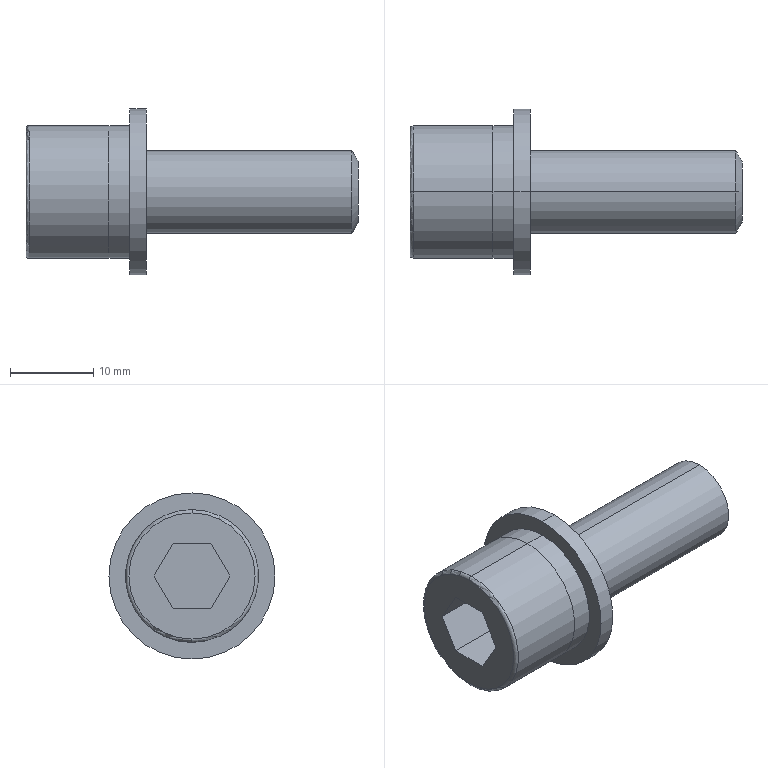Part | SolidWorks | features BaseBody 3 | 3 solids | 36 faces | box 40 x 20 x 20 mm | volume 4745 mm3 | plane 16 | cylinder 14 | torus 4 | cone 2 | commonest cylinder face diameters 16 x5 11 x3 10 x2 10.5 x2 20 x2
STEP:
#1=CARTESIAN_POINT('',(40.,0.,3.701));
#2=VERTEX_POINT('',#1);
#3=CARTESIAN_POINT('',(40.,0.,-3.701));
#4=VERTEX_POINT('',#3);
#5=CARTESIAN_POINT('',(40.,0.,0.));
#6=DIRECTION('',(-1.,0.,0.));
#7=DIRECTION('',(0.,0.,1.));
#8=AXIS2_PLACEMENT_3D('',#5,#6,#7);
#9=CIRCLE('',#8,3.701);
#10=EDGE_CURVE('',#2,#4,#9,.T.);
#11=ORIENTED_EDGE('',*,*,#10,.T.);
#12=CARTESIAN_POINT('',(39.25,0.,-5.));
#13=VERTEX_POINT('',#12);
#14=CARTESIAN_POINT('',(39.25,0.,-5.));
#15=DIRECTION('',(-0.5,0.,-0.866));
#16=VECTOR('',#15,1000.);
#17=LINE('',#14,#16);
#18=EDGE_CURVE('',#4,#13,#17,.T.);
#19=ORIENTED_EDGE('',*,*,#18,.T.);
#20=CARTESIAN_POINT('',(39.25,0.,5.));
#21=VERTEX_POINT('',#20);
#22=CARTESIAN_POINT('',(39.25,0.,0.));
#23=DIRECTION('',(-1.,0.,0.));
#24=DIRECTION('',(0.,0.,1.));
#25=AXIS2_PLACEMENT_3D('',#22,#23,#24);
#26=CIRCLE('',#25,5.);
#27=EDGE_CURVE('',#21,#13,#26,.T.);
#28=ORIENTED_EDGE('',*,*,#27,.F.);
#29=CARTESIAN_POINT('',(39.25,0.,5.));
#30=DIRECTION('',(-0.5,0.,0.866));
#31=VECTOR('',#30,1000.);
#32=LINE('',#29,#31);
#33=EDGE_CURVE('',#2,#21,#32,.T.);
#34=ORIENTED_EDGE('',*,*,#33,.F.);
#35=EDGE_LOOP('',(#11,#19,#28,#34));
#36=FACE_OUTER_BOUND('',#35,.T.);
#37=CARTESIAN_POINT('',(39.25,0.,0.));
#38=DIRECTION('',(-1.,0.,0.));
#39=DIRECTION('',(0.,0.,1.));
#40=AXIS2_PLACEMENT_3D('',#37,#38,#39);
#41=CONICAL_SURFACE('',#40,5.,1.047);
#42=ADVANCED_FACE('',(#36),#41,.T.);
#43=CARTESIAN_POINT('',(0.4,0.,-8.));
#44=VERTEX_POINT('',#43);
#45=CARTESIAN_POINT('',(0.4,0.,8.));
#46=VERTEX_POINT('',#45);
#47=CARTESIAN_POINT('',(0.4,0.,0.));
#48=DIRECTION('',(1.,0.,0.));
#49=DIRECTION('',(0.,0.,1.));
#50=AXIS2_PLACEMENT_3D('',#47,#48,#49);
#51=CIRCLE('',#50,8.);
#52=EDGE_CURVE('',#44,#46,#51,.T.);
#53=ORIENTED_EDGE('',*,*,#52,.F.);
#54=CARTESIAN_POINT('',(0.,0.,-7.6));
#55=VERTEX_POINT('',#54);
#56=CARTESIAN_POINT('',(0.4,0.,-7.6));
#57=DIRECTION('',(0.,1.,0.));
#58=DIRECTION('',(0.,0.,1.));
#59=AXIS2_PLACEMENT_3D('',#56,#57,#58);
#60=CIRCLE('',#59,0.4);
#61=EDGE_CURVE('',#44,#55,#60,.T.);
#62=ORIENTED_EDGE('',*,*,#61,.T.);
#63=CARTESIAN_POINT('',(0.,0.,7.6));
#64=VERTEX_POINT('',#63);
#65=CARTESIAN_POINT('',(0.,0.,0.));
#66=DIRECTION('',(-1.,0.,0.));
#67=DIRECTION('',(0.,0.,1.));
#68=AXIS2_PLACEMENT_3D('',#65,#66,#67);
#69=CIRCLE('',#68,7.6);
#70=EDGE_CURVE('',#64,#55,#69,.T.);
#71=ORIENTED_EDGE('',*,*,#70,.F.);
#72=CARTESIAN_POINT('',(0.4,0.,7.6));
#73=DIRECTION('',(0.,-1.,0.));
#74=DIRECTION('',(0.,0.,-1.));
#75=AXIS2_PLACEMENT_3D('',#72,#73,#74);
#76=CIRCLE('',#75,0.4);
#77=EDGE_CURVE('',#46,#64,#76,.T.);
#78=ORIENTED_EDGE('',*,*,#77,.F.);
#79=EDGE_LOOP('',(#53,#62,#71,#78));
#80=FACE_OUTER_BOUND('',#79,.T.);
#81=CARTESIAN_POINT('',(0.4,0.,0.));
#82=DIRECTION('',(-1.,0.,0.));
#83=DIRECTION('',(0.,0.,1.));
#84=AXIS2_PLACEMENT_3D('',#81,#82,#83);
#85=TOROIDAL_SURFACE('',#84,7.6,0.4);
#86=ADVANCED_FACE('',(#80),#85,.T.);
#87=CARTESIAN_POINT('',(10.4,0.,5.));
#88=VERTEX_POINT('',#87);
#89=CARTESIAN_POINT('',(10.4,0.,-5.));
#90=VERTEX_POINT('',#89);
#91=CARTESIAN_POINT('',(10.4,0.,0.));
#92=DIRECTION('',(1.,0.,0.));
#93=DIRECTION('',(0.,0.,-1.));
#94=AXIS2_PLACEMENT_3D('',#91,#92,#93);
#95=CIRCLE('',#94,5.);
#96=EDGE_CURVE('',#88,#90,#95,.T.);
#97=ORIENTED_EDGE('',*,*,#96,.F.);
#98=CARTESIAN_POINT('',(10.,0.,5.4));
#99=VERTEX_POINT('',#98);
#100=CARTESIAN_POINT('',(10.4,0.,5.4));
#101=DIRECTION('',(0.,1.,0.));
#102=DIRECTION('',(0.,0.,1.));
#103=AXIS2_PLACEMENT_3D('',#100,#101,#102);
#104=CIRCLE('',#103,0.4);
#105=EDGE_CURVE('',#88,#99,#104,.T.);
#106=ORIENTED_EDGE('',*,*,#105,.T.);
#107=CARTESIAN_POINT('',(10.,0.,-5.4));
#108=VERTEX_POINT('',#107);
#109=CARTESIAN_POINT('',(10.,0.,0.));
#110=DIRECTION('',(1.,0.,0.));
#111=DIRECTION('',(0.,0.,-1.));
#112=AXIS2_PLACEMENT_3D('',#109,#110,#111);
#113=CIRCLE('',#112,5.4);
#114=EDGE_CURVE('',#99,#108,#113,.T.);
#115=ORIENTED_EDGE('',*,*,#114,.T.);
#116=CARTESIAN_POINT('',(10.4,0.,-5.4));
#117=DIRECTION('',(0.,-1.,0.));
#118=DIRECTION('',(0.,0.,-1.));
#119=AXIS2_PLACEMENT_3D('',#116,#117,#118);
#120=CIRCLE('',#119,0.4);
#121=EDGE_CURVE('',#90,#108,#120,.T.);
#122=ORIENTED_EDGE('',*,*,#121,.F.);
#123=EDGE_LOOP('',(#97,#106,#115,#122));
#124=FACE_OUTER_BOUND('',#123,.T.);
#125=CARTESIAN_POINT('',(10.4,0.,0.));
#126=DIRECTION('',(1.,0.,0.));
#127=DIRECTION('',(0.,0.,-1.));
#128=AXIS2_PLACEMENT_3D('',#125,#126,#127);
#129=TOROIDAL_SURFACE('',#128,5.4,0.4);
#130=ADVANCED_FACE('',(#124),#129,.F.);
#131=ORIENTED_EDGE('',*,*,#52,.T.);
#132=CARTESIAN_POINT('',(10.,0.,8.));
#133=VERTEX_POINT('',#132);
#134=CARTESIAN_POINT('',(0.,0.,8.));
#135=DIRECTION('',(1.,0.,0.));
#136=VECTOR('',#135,1000.);
#137=LINE('',#134,#136);
#138=EDGE_CURVE('',#46,#133,#137,.T.);
#139=ORIENTED_EDGE('',*,*,#138,.T.);
#140=CARTESIAN_POINT('',(10.,0.,-8.));
#141=VERTEX_POINT('',#140);
#142=CARTESIAN_POINT('',(10.,0.,0.));
#143=DIRECTION('',(1.,0.,0.));
#144=DIRECTION('',(0.,0.,-1.));
#145=AXIS2_PLACEMENT_3D('',#142,#143,#144);
#146=CIRCLE('',#145,8.);
#147=EDGE_CURVE('',#141,#133,#146,.T.);
#148=ORIENTED_EDGE('',*,*,#147,.F.);
#149=CARTESIAN_POINT('',(0.,0.,-8.));
#150=DIRECTION('',(1.,0.,0.));
#151=VECTOR('',#150,1000.);
#152=LINE('',#149,#151);
#153=EDGE_CURVE('',#44,#141,#152,.T.);
#154=ORIENTED_EDGE('',*,*,#153,.F.);
#155=EDGE_LOOP('',(#131,#139,#148,#154));
#156=FACE_OUTER_BOUND('',#155,.T.);
#157=CARTESIAN_POINT('',(0.,0.,0.));
#158=DIRECTION('',(1.,0.,0.));
#159=DIRECTION('',(0.,0.,-1.));
#160=AXIS2_PLACEMENT_3D('',#157,#158,#159);
#161=CYLINDRICAL_SURFACE('',#160,8.);
#162=ADVANCED_FACE('',(#156),#161,.T.);
#163=CARTESIAN_POINT('',(10.4,0.,0.));
#164=DIRECTION('',(1.,0.,0.));
#165=DIRECTION('',(0.,0.,-1.));
#166=AXIS2_PLACEMENT_3D('',#163,#164,#165);
#167=CIRCLE('',#166,5.);
#168=EDGE_CURVE('',#90,#88,#167,.T.);
#169=ORIENTED_EDGE('',*,*,#168,.T.);
#170=CARTESIAN_POINT('',(0.,0.,5.));
#171=DIRECTION('',(1.,0.,0.));
#172=VECTOR('',#171,1000.);
#173=LINE('',#170,#172);
#174=EDGE_CURVE('',#88,#21,#173,.T.);
#175=ORIENTED_EDGE('',*,*,#174,.T.);
#176=ORIENTED_EDGE('',*,*,#27,.T.);
#177=CARTESIAN_POINT('',(0.,0.,-5.));
#178=DIRECTION('',(1.,0.,0.));
#179=VECTOR('',#178,1000.);
#180=LINE('',#177,#179);
#181=EDGE_CURVE('',#90,#13,#180,.T.);
#182=ORIENTED_EDGE('',*,*,#181,.F.);
#183=EDGE_LOOP('',(#169,#175,#176,#182));
#184=FACE_OUTER_BOUND('',#183,.T.);
#185=CARTESIAN_POINT('',(0.,0.,0.));
#186=DIRECTION('',(1.,0.,0.));
#187=DIRECTION('',(0.,0.,-1.));
#188=AXIS2_PLACEMENT_3D('',#185,#186,#187);
#189=CYLINDRICAL_SURFACE('',#188,5.);
#190=ADVANCED_FACE('',(#184),#189,.T.);
#191=ORIENTED_EDGE('',*,*,#174,.F.);
#192=ORIENTED_EDGE('',*,*,#96,.T.);
#193=ORIENTED_EDGE('',*,*,#181,.T.);
#194=CARTESIAN_POINT('',(39.25,0.,0.));
#195=DIRECTION('',(-1.,0.,0.));
#196=DIRECTION('',(0.,0.,1.));
#197=AXIS2_PLACEMENT_3D('',#194,#195,#196);
#198=CIRCLE('',#197,5.);
#199=EDGE_CURVE('',#13,#21,#198,.T.);
#200=ORIENTED_EDGE('',*,*,#199,.T.);
#201=EDGE_LOOP('',(#191,#192,#193,#200));
#202=FACE_OUTER_BOUND('',#201,.T.);
#203=CARTESIAN_POINT('',(0.,0.,0.));
#204=DIRECTION('',(1.,0.,0.));
#205=DIRECTION('',(0.,0.,-1.));
#206=AXIS2_PLACEMENT_3D('',#203,#204,#205);
#207=CYLINDRICAL_SURFACE('',#206,5.);
#208=ADVANCED_FACE('',(#202),#207,.T.);
#209=ORIENTED_EDGE('',*,*,#70,.T.);
#210=CARTESIAN_POINT('',(0.,0.,0.));
#211=DIRECTION('',(-1.,0.,0.));
#212=DIRECTION('',(0.,0.,1.));
#213=AXIS2_PLACEMENT_3D('',#210,#211,#212);
#214=CIRCLE('',#213,7.6);
#215=EDGE_CURVE('',#55,#64,#214,.T.);
#216=ORIENTED_EDGE('',*,*,#215,.T.);
#217=EDGE_LOOP('',(#209,#216));
#218=FACE_OUTER_BOUND('',#217,.T.);
#219=CARTESIAN_POINT('',(0.,-4.575,0.));
#220=VERTEX_POINT('',#219);
#221=CARTESIAN_POINT('',(0.,-2.288,3.962));
#222=VERTEX_POINT('',#221);
#223=CARTESIAN_POINT('',(0.,-4.575,0.));
#224=DIRECTION('',(0.,0.5,0.866));
#225=VECTOR('',#224,1000.);
#226=LINE('',#223,#225);
#227=EDGE_CURVE('',#220,#222,#226,.T.);
#228=ORIENTED_EDGE('',*,*,#227,.F.);
#229=CARTESIAN_POINT('',(0.,-2.288,-3.962));
#230=VERTEX_POINT('',#229);
#231=CARTESIAN_POINT('',(0.,-2.288,-3.962));
#232=DIRECTION('',(0.,-0.5,0.866));
#233=VECTOR('',#232,1000.);
#234=LINE('',#231,#233);
#235=EDGE_CURVE('',#230,#220,#234,.T.);
#236=ORIENTED_EDGE('',*,*,#235,.F.);
#237=CARTESIAN_POINT('',(0.,2.288,-3.962));
#238=VERTEX_POINT('',#237);
#239=CARTESIAN_POINT('',(0.,2.288,-3.962));
#240=DIRECTION('',(0.,-1.,0.));
#241=VECTOR('',#240,1000.);
#242=LINE('',#239,#241);
#243=EDGE_CURVE('',#238,#230,#242,.T.);
#244=ORIENTED_EDGE('',*,*,#243,.F.);
#245=CARTESIAN_POINT('',(0.,4.575,0.));
#246=VERTEX_POINT('',#245);
#247=CARTESIAN_POINT('',(0.,4.575,0.));
#248=DIRECTION('',(0.,-0.5,-0.866));
#249=VECTOR('',#248,1000.);
#250=LINE('',#247,#249);
#251=EDGE_CURVE('',#246,#238,#250,.T.);
#252=ORIENTED_EDGE('',*,*,#251,.F.);
#253=CARTESIAN_POINT('',(0.,2.288,3.962));
#254=VERTEX_POINT('',#253);
#255=CARTESIAN_POINT('',(0.,2.288,3.962));
#256=DIRECTION('',(0.,0.5,-0.866));
#257=VECTOR('',#256,1000.);
#258=LINE('',#255,#257);
#259=EDGE_CURVE('',#254,#246,#258,.T.);
#260=ORIENTED_EDGE('',*,*,#259,.F.);
#261=CARTESIAN_POINT('',(0.,-2.288,3.962));
#262=DIRECTION('',(0.,1.,0.));
#263=VECTOR('',#262,1000.);
#264=LINE('',#261,#263);
#265=EDGE_CURVE('',#222,#254,#264,.T.);
#266=ORIENTED_EDGE('',*,*,#265,.F.);
#267=EDGE_LOOP('',(#228,#236,#244,#252,#260,#266));
#268=FACE_BOUND('',#267,.T.);
#269=CARTESIAN_POINT('',(0.,0.,0.));
#270=DIRECTION('',(-1.,0.,0.));
#271=DIRECTION('',(0.,0.,1.));
#272=AXIS2_PLACEMENT_3D('',#269,#270,#271);
#273=PLANE('',#272);
#274=ADVANCED_FACE('',(#218,#268),#273,.T.);
#275=ORIENTED_EDGE('',*,*,#138,.F.);
#276=CARTESIAN_POINT('',(0.4,0.,0.));
#277=DIRECTION('',(1.,0.,0.));
#278=DIRECTION('',(0.,0.,1.));
#279=AXIS2_PLACEMENT_3D('',#276,#277,#278);
#280=CIRCLE('',#279,8.);
#281=EDGE_CURVE('',#46,#44,#280,.T.);
#282=ORIENTED_EDGE('',*,*,#281,.T.);
#283=ORIENTED_EDGE('',*,*,#153,.T.);
#284=CARTESIAN_POINT('',(10.,0.,0.));
#285=DIRECTION('',(1.,0.,0.));
#286=DIRECTION('',(0.,0.,-1.));
#287=AXIS2_PLACEMENT_3D('',#284,#285,#286);
#288=CIRCLE('',#287,8.);
#289=EDGE_CURVE('',#133,#141,#288,.T.);
#290=ORIENTED_EDGE('',*,*,#289,.F.);
#291=EDGE_LOOP('',(#275,#282,#283,#290));
#292=FACE_OUTER_BOUND('',#291,.T.);
#293=CARTESIAN_POINT('',(0.,0.,0.));
#294=DIRECTION('',(1.,0.,0.));
#295=DIRECTION('',(0.,0.,-1.));
#296=AXIS2_PLACEMENT_3D('',#293,#294,#295);
#297=CYLINDRICAL_SURFACE('',#296,8.);
#298=ADVANCED_FACE('',(#292),#297,.T.);
#299=ORIENTED_EDGE('',*,*,#147,.T.);
#300=ORIENTED_EDGE('',*,*,#289,.T.);
#301=EDGE_LOOP('',(#299,#300));
#302=FACE_OUTER_BOUND('',#301,.T.);
#303=CARTESIAN_POINT('',(10.,0.,0.));
#304=DIRECTION('',(1.,0.,0.));
#305=DIRECTION('',(0.,0.,-1.));
#306=AXIS2_PLACEMENT_3D('',#303,#304,#305);
#307=CIRCLE('',#306,5.4);
#308=EDGE_CURVE('',#108,#99,#307,.T.);
#309=ORIENTED_EDGE('',*,*,#308,.F.);
#310=ORIENTED_EDGE('',*,*,#114,.F.);
#311=EDGE_LOOP('',(#309,#310));
#312=FACE_BOUND('',#311,.T.);
#313=CARTESIAN_POINT('',(10.,8.,0.));
#314=DIRECTION('',(1.,0.,0.));
#315=DIRECTION('',(0.,0.,-1.));
#316=AXIS2_PLACEMENT_3D('',#313,#314,#315);
#317=PLANE('',#316);
#318=ADVANCED_FACE('',(#302,#312),#317,.T.);
#319=ORIENTED_EDGE('',*,*,#105,.F.);
#320=ORIENTED_EDGE('',*,*,#168,.F.);
#321=ORIENTED_EDGE('',*,*,#121,.T.);
#322=ORIENTED_EDGE('',*,*,#308,.T.);
#323=EDGE_LOOP('',(#319,#320,#321,#322));
#324=FACE_OUTER_BOUND('',#323,.T.);
#325=CARTESIAN_POINT('',(10.4,0.,0.));
#326=DIRECTION('',(1.,0.,0.));
#327=DIRECTION('',(0.,0.,-1.));
#328=AXIS2_PLACEMENT_3D('',#325,#326,#327);
#329=TOROIDAL_SURFACE('',#328,5.4,0.4);
#330=ADVANCED_FACE('',(#324),#329,.F.);
#331=ORIENTED_EDGE('',*,*,#227,.T.);
#332=CARTESIAN_POINT('',(6.,-2.288,3.962));
#333=VERTEX_POINT('',#332);
#334=CARTESIAN_POINT('',(6.,-2.288,3.962));
#335=DIRECTION('',(-1.,0.,0.));
#336=VECTOR('',#335,1000.);
#337=LINE('',#334,#336);
#338=EDGE_CURVE('',#333,#222,#337,.T.);
#339=ORIENTED_EDGE('',*,*,#338,.F.);
#340=CARTESIAN_POINT('',(6.,-4.575,0.));
#341=VERTEX_POINT('',#340);
#342=CARTESIAN_POINT('',(6.,-4.575,0.));
#343=DIRECTION('',(0.,0.5,0.866));
#344=VECTOR('',#343,1000.);
#345=LINE('',#342,#344);
#346=EDGE_CURVE('',#341,#333,#345,.T.);
#347=ORIENTED_EDGE('',*,*,#346,.F.);
#348=CARTESIAN_POINT('',(6.,-4.575,0.));
#349=DIRECTION('',(-1.,0.,0.));
#350=VECTOR('',#349,1000.);
#351=LINE('',#348,#350);
#352=EDGE_CURVE('',#341,#220,#351,.T.);
#353=ORIENTED_EDGE('',*,*,#352,.T.);
#354=EDGE_LOOP('',(#331,#339,#347,#353));
#355=FACE_OUTER_BOUND('',#354,.T.);
#356=CARTESIAN_POINT('',(6.,-4.575,0.));
#357=DIRECTION('',(0.,-0.866,0.5));
#358=DIRECTION('',(0.,-0.5,-0.866));
#359=AXIS2_PLACEMENT_3D('',#356,#357,#358);
#360=PLANE('',#359);
#361=ADVANCED_FACE('',(#355),#360,.F.);
#362=ORIENTED_EDGE('',*,*,#235,.T.);
#363=ORIENTED_EDGE('',*,*,#352,.F.);
#364=CARTESIAN_POINT('',(6.,-2.288,-3.962));
#365=VERTEX_POINT('',#364);
#366=CARTESIAN_POINT('',(6.,-2.288,-3.962));
#367=DIRECTION('',(0.,-0.5,0.866));
#368=VECTOR('',#367,1000.);
#369=LINE('',#366,#368);
#370=EDGE_CURVE('',#365,#341,#369,.T.);
#371=ORIENTED_EDGE('',*,*,#370,.F.);
#372=CARTESIAN_POINT('',(6.,-2.288,-3.962));
#373=DIRECTION('',(-1.,0.,0.));
#374=VECTOR('',#373,1000.);
#375=LINE('',#372,#374);
#376=EDGE_CURVE('',#365,#230,#375,.T.);
#377=ORIENTED_EDGE('',*,*,#376,.T.);
#378=EDGE_LOOP('',(#362,#363,#371,#377));
#379=FACE_OUTER_BOUND('',#378,.T.);
#380=CARTESIAN_POINT('',(6.,-2.288,-3.962));
#381=DIRECTION('',(0.,-0.866,-0.5));
#382=DIRECTION('',(0.,0.5,-0.866));
#383=AXIS2_PLACEMENT_3D('',#380,#381,#382);
#384=PLANE('',#383);
#385=ADVANCED_FACE('',(#379),#384,.F.);
#386=ORIENTED_EDGE('',*,*,#243,.T.);
#387=ORIENTED_EDGE('',*,*,#376,.F.);
#388=CARTESIAN_POINT('',(6.,2.288,-3.962));
#389=VERTEX_POINT('',#388);
#390=CARTESIAN_POINT('',(6.,2.288,-3.962));
#391=DIRECTION('',(0.,-1.,0.));
#392=VECTOR('',#391,1000.);
#393=LINE('',#390,#392);
#394=EDGE_CURVE('',#389,#365,#393,.T.);
#395=ORIENTED_EDGE('',*,*,#394,.F.);
#396=CARTESIAN_POINT('',(6.,2.288,-3.962));
#397=DIRECTION('',(-1.,0.,0.));
#398=VECTOR('',#397,1000.);
#399=LINE('',#396,#398);
#400=EDGE_CURVE('',#389,#238,#399,.T.);
#401=ORIENTED_EDGE('',*,*,#400,.T.);
#402=EDGE_LOOP('',(#386,#387,#395,#401));
#403=FACE_OUTER_BOUND('',#402,.T.);
#404=CARTESIAN_POINT('',(6.,2.288,-3.962));
#405=DIRECTION('',(0.,0.,-1.));
#406=DIRECTION('',(0.,1.,0.));
#407=AXIS2_PLACEMENT_3D('',#404,#405,#406);
#408=PLANE('',#407);
#409=ADVANCED_FACE('',(#403),#408,.F.);
#410=ORIENTED_EDGE('',*,*,#251,.T.);
#411=ORIENTED_EDGE('',*,*,#400,.F.);
#412=CARTESIAN_POINT('',(6.,4.575,0.));
#413=VERTEX_POINT('',#412);
#414=CARTESIAN_POINT('',(6.,4.575,0.));
#415=DIRECTION('',(0.,-0.5,-0.866));
#416=VECTOR('',#415,1000.);
#417=LINE('',#414,#416);
#418=EDGE_CURVE('',#413,#389,#417,.T.);
#419=ORIENTED_EDGE('',*,*,#418,.F.);
#420=CARTESIAN_POINT('',(6.,4.575,0.));
#421=DIRECTION('',(-1.,0.,0.));
#422=VECTOR('',#421,1000.);
#423=LINE('',#420,#422);
#424=EDGE_CURVE('',#413,#246,#423,.T.);
#425=ORIENTED_EDGE('',*,*,#424,.T.);
#426=EDGE_LOOP('',(#410,#411,#419,#425));
#427=FACE_OUTER_BOUND('',#426,.T.);
#428=CARTESIAN_POINT('',(6.,4.575,0.));
#429=DIRECTION('',(0.,0.866,-0.5));
#430=DIRECTION('',(0.,0.5,0.866));
#431=AXIS2_PLACEMENT_3D('',#428,#429,#430);
#432=PLANE('',#431);
#433=ADVANCED_FACE('',(#427),#432,.F.);
#434=ORIENTED_EDGE('',*,*,#259,.T.);
#435=ORIENTED_EDGE('',*,*,#424,.F.);
#436=CARTESIAN_POINT('',(6.,2.288,3.962));
#437=VERTEX_POINT('',#436);
#438=CARTESIAN_POINT('',(6.,2.288,3.962));
#439=DIRECTION('',(0.,0.5,-0.866));
#440=VECTOR('',#439,1000.);
#441=LINE('',#438,#440);
#442=EDGE_CURVE('',#437,#413,#441,.T.);
#443=ORIENTED_EDGE('',*,*,#442,.F.);
#444=CARTESIAN_POINT('',(6.,2.288,3.962));
#445=DIRECTION('',(-1.,0.,0.));
#446=VECTOR('',#445,1000.);
#447=LINE('',#444,#446);
#448=EDGE_CURVE('',#437,#254,#447,.T.);
#449=ORIENTED_EDGE('',*,*,#448,.T.);
#450=EDGE_LOOP('',(#434,#435,#443,#449));
#451=FACE_OUTER_BOUND('',#450,.T.);
#452=CARTESIAN_POINT('',(6.,2.288,3.962));
#453=DIRECTION('',(0.,0.866,0.5));
#454=DIRECTION('',(0.,-0.5,0.866));
#455=AXIS2_PLACEMENT_3D('',#452,#453,#454);
#456=PLANE('',#455);
#457=ADVANCED_FACE('',(#451),#456,.F.);
#458=ORIENTED_EDGE('',*,*,#265,.T.);
#459=ORIENTED_EDGE('',*,*,#448,.F.);
#460=CARTESIAN_POINT('',(6.,-2.288,3.962));
#461=DIRECTION('',(0.,1.,0.));
#462=VECTOR('',#461,1000.);
#463=LINE('',#460,#462);
#464=EDGE_CURVE('',#333,#437,#463,.T.);
#465=ORIENTED_EDGE('',*,*,#464,.F.);
#466=ORIENTED_EDGE('',*,*,#338,.T.);
#467=EDGE_LOOP('',(#458,#459,#465,#466));
#468=FACE_OUTER_BOUND('',#467,.T.);
#469=CARTESIAN_POINT('',(6.,-2.288,3.962));
#470=DIRECTION('',(0.,0.,1.));
#471=DIRECTION('',(0.,-1.,0.));
#472=AXIS2_PLACEMENT_3D('',#469,#470,#471);
#473=PLANE('',#472);
#474=ADVANCED_FACE('',(#468),#473,.F.);
#475=ORIENTED_EDGE('',*,*,#346,.T.);
#476=ORIENTED_EDGE('',*,*,#464,.T.);
#477=ORIENTED_EDGE('',*,*,#442,.T.);
#478=ORIENTED_EDGE('',*,*,#418,.T.);
#479=ORIENTED_EDGE('',*,*,#394,.T.);
#480=ORIENTED_EDGE('',*,*,#370,.T.);
#481=EDGE_LOOP('',(#475,#476,#477,#478,#479,#480));
#482=FACE_OUTER_BOUND('',#481,.T.);
#483=CARTESIAN_POINT('',(6.,-2.288,3.962));
#484=DIRECTION('',(-1.,0.,0.));
#485=DIRECTION('',(0.,0.,1.));
#486=AXIS2_PLACEMENT_3D('',#483,#484,#485);
#487=PLANE('',#486);
#488=ADVANCED_FACE('',(#482),#487,.T.);
#489=ORIENTED_EDGE('',*,*,#61,.F.);
#490=ORIENTED_EDGE('',*,*,#281,.F.);
#491=ORIENTED_EDGE('',*,*,#77,.T.);
#492=ORIENTED_EDGE('',*,*,#215,.F.);
#493=EDGE_LOOP('',(#489,#490,#491,#492));
#494=FACE_OUTER_BOUND('',#493,.T.);
#495=CARTESIAN_POINT('',(0.4,0.,0.));
#496=DIRECTION('',(-1.,0.,0.));
#497=DIRECTION('',(0.,0.,1.));
#498=AXIS2_PLACEMENT_3D('',#495,#496,#497);
#499=TOROIDAL_SURFACE('',#498,7.6,0.4);
#500=ADVANCED_FACE('',(#494),#499,.T.);
#501=ORIENTED_EDGE('',*,*,#18,.F.);
#502=CARTESIAN_POINT('',(40.,0.,0.));
#503=DIRECTION('',(-1.,0.,0.));
#504=DIRECTION('',(0.,0.,1.));
#505=AXIS2_PLACEMENT_3D('',#502,#503,#504);
#506=CIRCLE('',#505,3.701);
#507=EDGE_CURVE('',#4,#2,#506,.T.);
#508=ORIENTED_EDGE('',*,*,#507,.T.);
#509=ORIENTED_EDGE('',*,*,#33,.T.);
#510=ORIENTED_EDGE('',*,*,#199,.F.);
#511=EDGE_LOOP('',(#501,#508,#509,#510));
#512=FACE_OUTER_BOUND('',#511,.T.);
#513=CARTESIAN_POINT('',(39.25,0.,0.));
#514=DIRECTION('',(-1.,0.,0.));
#515=DIRECTION('',(0.,0.,1.));
#516=AXIS2_PLACEMENT_3D('',#513,#514,#515);
#517=CONICAL_SURFACE('',#516,5.,1.047);
#518=ADVANCED_FACE('',(#512),#517,.T.);
#519=ORIENTED_EDGE('',*,*,#10,.F.);
#520=ORIENTED_EDGE('',*,*,#507,.F.);
#521=EDGE_LOOP('',(#519,#520));
#522=FACE_OUTER_BOUND('',#521,.T.);
#523=CARTESIAN_POINT('',(40.,5.,0.));
#524=DIRECTION('',(1.,0.,0.));
#525=DIRECTION('',(0.,0.,-1.));
#526=AXIS2_PLACEMENT_3D('',#523,#524,#525);
#527=PLANE('',#526);
#528=ADVANCED_FACE('',(#522),#527,.T.);
#529=CLOSED_SHELL('',(#42,#86,#130,#162,#190,#208,#274,#298,#318,#330,#361,#385,#409,#433,#457,#474,#488,#500,#518,#528));
#530=MANIFOLD_SOLID_BREP('',#529);
#531=CARTESIAN_POINT('',(12.5,0.,-8.));
#532=VERTEX_POINT('',#531);
#533=CARTESIAN_POINT('',(12.5,7.862,-1.479));
#534=VERTEX_POINT('',#533);
#535=CARTESIAN_POINT('',(12.5,0.,0.));
#536=DIRECTION('',(1.,0.,0.));
#537=DIRECTION('',(0.,0.,-1.));
#538=AXIS2_PLACEMENT_3D('',#535,#536,#537);
#539=CIRCLE('',#538,8.);
#540=EDGE_CURVE('',#532,#534,#539,.T.);
#541=ORIENTED_EDGE('',*,*,#540,.F.);
#542=CARTESIAN_POINT('',(10.,0.,-8.));
#543=VERTEX_POINT('',#542);
#544=CARTESIAN_POINT('',(12.5,0.,-8.));
#545=DIRECTION('',(-1.,0.,0.));
#546=VECTOR('',#545,1000.);
#547=LINE('',#544,#546);
#548=EDGE_CURVE('',#532,#543,#547,.T.);
#549=ORIENTED_EDGE('',*,*,#548,.T.);
#550=CARTESIAN_POINT('',(10.,7.862,-1.479));
#551=VERTEX_POINT('',#550);
#552=CARTESIAN_POINT('',(10.,0.,0.));
#553=DIRECTION('',(1.,0.,0.));
#554=DIRECTION('',(0.,0.,-1.));
#555=AXIS2_PLACEMENT_3D('',#552,#553,#554);
#556=CIRCLE('',#555,8.);
#557=EDGE_CURVE('',#543,#551,#556,.T.);
#558=ORIENTED_EDGE('',*,*,#557,.T.);
#559=CARTESIAN_POINT('',(12.5,7.862,-1.479));
#560=DIRECTION('',(-1.,0.,0.));
#561=VECTOR('',#560,1000.);
#562=LINE('',#559,#561);
#563=EDGE_CURVE('',#534,#551,#562,.T.);
#564=ORIENTED_EDGE('',*,*,#563,.F.);
#565=EDGE_LOOP('',(#541,#549,#558,#564));
#566=FACE_OUTER_BOUND('',#565,.T.);
#567=CARTESIAN_POINT('',(12.5,0.,0.));
#568=DIRECTION('',(-1.,0.,0.));
#569=DIRECTION('',(0.,0.,1.));
#570=AXIS2_PLACEMENT_3D('',#567,#568,#569);
#571=CYLINDRICAL_SURFACE('',#570,8.);
#572=ADVANCED_FACE('',(#566),#571,.T.);
#573=ORIENTED_EDGE('',*,*,#548,.F.);
#574=CARTESIAN_POINT('',(12.5,0.,8.));
#575=VERTEX_POINT('',#574);
#576=CARTESIAN_POINT('',(12.5,0.,0.));
#577=DIRECTION('',(1.,0.,0.));
#578=DIRECTION('',(0.,0.,-1.));
#579=AXIS2_PLACEMENT_3D('',#576,#577,#578);
#580=CIRCLE('',#579,8.);
#581=EDGE_CURVE('',#575,#532,#580,.T.);
#582=ORIENTED_EDGE('',*,*,#581,.F.);
#583=CARTESIAN_POINT('',(10.,0.,8.));
#584=VERTEX_POINT('',#583);
#585=CARTESIAN_POINT('',(12.5,0.,8.));
#586=DIRECTION('',(-1.,0.,0.));
#587=VECTOR('',#586,1000.);
#588=LINE('',#585,#587);
#589=EDGE_CURVE('',#575,#584,#588,.T.);
#590=ORIENTED_EDGE('',*,*,#589,.T.);
#591=CARTESIAN_POINT('',(10.,0.,0.));
#592=DIRECTION('',(1.,0.,0.));
#593=DIRECTION('',(0.,0.,-1.));
#594=AXIS2_PLACEMENT_3D('',#591,#592,#593);
#595=CIRCLE('',#594,8.);
#596=EDGE_CURVE('',#584,#543,#595,.T.);
#597=ORIENTED_EDGE('',*,*,#596,.T.);
#598=EDGE_LOOP('',(#573,#582,#590,#597));
#599=FACE_OUTER_BOUND('',#598,.T.);
#600=CARTESIAN_POINT('',(12.5,0.,0.));
#601=DIRECTION('',(-1.,0.,0.));
#602=DIRECTION('',(0.,0.,1.));
#603=AXIS2_PLACEMENT_3D('',#600,#601,#602);
#604=CYLINDRICAL_SURFACE('',#603,8.);
#605=ADVANCED_FACE('',(#599),#604,.T.);
#606=CARTESIAN_POINT('',(12.5,0.,-5.5));
#607=VERTEX_POINT('',#606);
#608=CARTESIAN_POINT('',(12.5,0.,5.5));
#609=VERTEX_POINT('',#608);
#610=CARTESIAN_POINT('',(12.5,0.,0.));
#611=DIRECTION('',(-1.,0.,0.));
#612=DIRECTION('',(0.,0.,-1.));
#613=AXIS2_PLACEMENT_3D('',#610,#611,#612);
#614=CIRCLE('',#613,5.5);
#615=EDGE_CURVE('',#607,#609,#614,.T.);
#616=ORIENTED_EDGE('',*,*,#615,.F.);
#617=CARTESIAN_POINT('',(10.,0.,-5.5));
#618=VERTEX_POINT('',#617);
#619=CARTESIAN_POINT('',(12.5,0.,-5.5));
#620=DIRECTION('',(-1.,0.,0.));
#621=VECTOR('',#620,1000.);
#622=LINE('',#619,#621);
#623=EDGE_CURVE('',#607,#618,#622,.T.);
#624=ORIENTED_EDGE('',*,*,#623,.T.);
#625=CARTESIAN_POINT('',(10.,0.,5.5));
#626=VERTEX_POINT('',#625);
#627=CARTESIAN_POINT('',(10.,0.,0.));
#628=DIRECTION('',(-1.,0.,0.));
#629=DIRECTION('',(0.,0.,-1.));
#630=AXIS2_PLACEMENT_3D('',#627,#628,#629);
#631=CIRCLE('',#630,5.5);
#632=EDGE_CURVE('',#618,#626,#631,.T.);
#633=ORIENTED_EDGE('',*,*,#632,.T.);
#634=CARTESIAN_POINT('',(12.5,0.,5.5));
#635=DIRECTION('',(-1.,0.,0.));
#636=VECTOR('',#635,1000.);
#637=LINE('',#634,#636);
#638=EDGE_CURVE('',#609,#626,#637,.T.);
#639=ORIENTED_EDGE('',*,*,#638,.F.);
#640=EDGE_LOOP('',(#616,#624,#633,#639));
#641=FACE_OUTER_BOUND('',#640,.T.);
#642=CARTESIAN_POINT('',(12.5,0.,0.));
#643=DIRECTION('',(-1.,0.,0.));
#644=DIRECTION('',(0.,0.,1.));
#645=AXIS2_PLACEMENT_3D('',#642,#643,#644);
#646=CYLINDRICAL_SURFACE('',#645,5.5);
#647=ADVANCED_FACE('',(#641),#646,.F.);
#648=CARTESIAN_POINT('',(12.5,5.499,0.1162));
#649=VERTEX_POINT('',#648);
#650=CARTESIAN_POINT('',(12.5,0.,0.));
#651=DIRECTION('',(-1.,0.,0.));
#652=DIRECTION('',(0.,0.,-1.));
#653=AXIS2_PLACEMENT_3D('',#650,#651,#652);
#654=CIRCLE('',#653,5.5);
#655=EDGE_CURVE('',#609,#649,#654,.T.);
#656=ORIENTED_EDGE('',*,*,#655,.F.);
#657=ORIENTED_EDGE('',*,*,#638,.T.);
#658=CARTESIAN_POINT('',(10.,5.499,0.1162));
#659=VERTEX_POINT('',#658);
#660=CARTESIAN_POINT('',(10.,0.,0.));
#661=DIRECTION('',(-1.,0.,0.));
#662=DIRECTION('',(0.,0.,-1.));
#663=AXIS2_PLACEMENT_3D('',#660,#661,#662);
#664=CIRCLE('',#663,5.5);
#665=EDGE_CURVE('',#626,#659,#664,.T.);
#666=ORIENTED_EDGE('',*,*,#665,.T.);
#667=CARTESIAN_POINT('',(12.5,5.499,0.1162));
#668=DIRECTION('',(-1.,0.,0.));
#669=VECTOR('',#668,1000.);
#670=LINE('',#667,#669);
#671=EDGE_CURVE('',#649,#659,#670,.T.);
#672=ORIENTED_EDGE('',*,*,#671,.F.);
#673=EDGE_LOOP('',(#656,#657,#666,#672));
#674=FACE_OUTER_BOUND('',#673,.T.);
#675=CARTESIAN_POINT('',(12.5,0.,0.));
#676=DIRECTION('',(-1.,0.,0.));
#677=DIRECTION('',(0.,0.,1.));
#678=AXIS2_PLACEMENT_3D('',#675,#676,#677);
#679=CYLINDRICAL_SURFACE('',#678,5.5);
#680=ADVANCED_FACE('',(#674),#679,.F.);
#681=ORIENTED_EDGE('',*,*,#623,.F.);
#682=CARTESIAN_POINT('',(12.5,5.499,-0.1148));
#683=VERTEX_POINT('',#682);
#684=CARTESIAN_POINT('',(12.5,0.,0.));
#685=DIRECTION('',(-1.,0.,0.));
#686=DIRECTION('',(0.,0.,-1.));
#687=AXIS2_PLACEMENT_3D('',#684,#685,#686);
#688=CIRCLE('',#687,5.5);
#689=EDGE_CURVE('',#683,#607,#688,.T.);
#690=ORIENTED_EDGE('',*,*,#689,.F.);
#691=CARTESIAN_POINT('',(10.,5.499,-0.1148));
#692=VERTEX_POINT('',#691);
#693=CARTESIAN_POINT('',(12.5,5.499,-0.1148));
#694=DIRECTION('',(-1.,0.,0.));
#695=VECTOR('',#694,1000.);
#696=LINE('',#693,#695);
#697=EDGE_CURVE('',#683,#692,#696,.T.);
#698=ORIENTED_EDGE('',*,*,#697,.T.);
#699=CARTESIAN_POINT('',(10.,0.,0.));
#700=DIRECTION('',(-1.,0.,0.));
#701=DIRECTION('',(0.,0.,-1.));
#702=AXIS2_PLACEMENT_3D('',#699,#700,#701);
#703=CIRCLE('',#702,5.5);
#704=EDGE_CURVE('',#692,#618,#703,.T.);
#705=ORIENTED_EDGE('',*,*,#704,.T.);
#706=EDGE_LOOP('',(#681,#690,#698,#705));
#707=FACE_OUTER_BOUND('',#706,.T.);
#708=CARTESIAN_POINT('',(12.5,0.,0.));
#709=DIRECTION('',(-1.,0.,0.));
#710=DIRECTION('',(0.,0.,1.));
#711=AXIS2_PLACEMENT_3D('',#708,#709,#710);
#712=CYLINDRICAL_SURFACE('',#711,5.5);
#713=ADVANCED_FACE('',(#707),#712,.F.);
#714=CARTESIAN_POINT('',(10.,7.899,-1.269));
#715=VERTEX_POINT('',#714);
#716=CARTESIAN_POINT('',(10.,5.499,0.1162));
#717=DIRECTION('',(0.,0.866,-0.5));
#718=VECTOR('',#717,1000.);
#719=LINE('',#716,#718);
#720=EDGE_CURVE('',#659,#715,#719,.T.);
#721=ORIENTED_EDGE('',*,*,#720,.T.);
#722=CARTESIAN_POINT('',(12.5,7.899,-1.269));
#723=VERTEX_POINT('',#722);
#724=CARTESIAN_POINT('',(12.5,7.899,-1.269));
#725=DIRECTION('',(-1.,0.,0.));
#726=VECTOR('',#725,1000.);
#727=LINE('',#724,#726);
#728=EDGE_CURVE('',#723,#715,#727,.T.);
#729=ORIENTED_EDGE('',*,*,#728,.F.);
#730=CARTESIAN_POINT('',(12.5,5.499,0.1162));
#731=DIRECTION('',(0.,0.866,-0.5));
#732=VECTOR('',#731,1000.);
#733=LINE('',#730,#732);
#734=EDGE_CURVE('',#649,#723,#733,.T.);
#735=ORIENTED_EDGE('',*,*,#734,.F.);
#736=ORIENTED_EDGE('',*,*,#671,.T.);
#737=EDGE_LOOP('',(#721,#729,#735,#736));
#738=FACE_OUTER_BOUND('',#737,.T.);
#739=CARTESIAN_POINT('',(12.5,5.499,0.1162));
#740=DIRECTION('',(0.,0.5,0.866));
#741=DIRECTION('',(0.,-0.866,0.5));
#742=AXIS2_PLACEMENT_3D('',#739,#740,#741);
#743=PLANE('',#742);
#744=ADVANCED_FACE('',(#738),#743,.F.);
#745=ORIENTED_EDGE('',*,*,#589,.F.);
#746=CARTESIAN_POINT('',(12.5,0.,0.));
#747=DIRECTION('',(1.,0.,0.));
#748=DIRECTION('',(0.,0.,-1.));
#749=AXIS2_PLACEMENT_3D('',#746,#747,#748);
#750=CIRCLE('',#749,8.);
#751=EDGE_CURVE('',#723,#575,#750,.T.);
#752=ORIENTED_EDGE('',*,*,#751,.F.);
#753=ORIENTED_EDGE('',*,*,#728,.T.);
#754=CARTESIAN_POINT('',(10.,0.,0.));
#755=DIRECTION('',(1.,0.,0.));
#756=DIRECTION('',(0.,0.,-1.));
#757=AXIS2_PLACEMENT_3D('',#754,#755,#756);
#758=CIRCLE('',#757,8.);
#759=EDGE_CURVE('',#715,#584,#758,.T.);
#760=ORIENTED_EDGE('',*,*,#759,.T.);
#761=EDGE_LOOP('',(#745,#752,#753,#760));
#762=FACE_OUTER_BOUND('',#761,.T.);
#763=CARTESIAN_POINT('',(12.5,0.,0.));
#764=DIRECTION('',(-1.,0.,0.));
#765=DIRECTION('',(0.,0.,1.));
#766=AXIS2_PLACEMENT_3D('',#763,#764,#765);
#767=CYLINDRICAL_SURFACE('',#766,8.);
#768=ADVANCED_FACE('',(#762),#767,.T.);
#769=CARTESIAN_POINT('',(10.,5.499,-0.1148));
#770=DIRECTION('',(0.,-0.866,0.5));
#771=VECTOR('',#770,1000.);
#772=LINE('',#769,#771);
#773=EDGE_CURVE('',#551,#692,#772,.T.);
#774=ORIENTED_EDGE('',*,*,#773,.T.);
#775=ORIENTED_EDGE('',*,*,#697,.F.);
#776=CARTESIAN_POINT('',(12.5,5.499,-0.1148));
#777=DIRECTION('',(0.,-0.866,0.5));
#778=VECTOR('',#777,1000.);
#779=LINE('',#776,#778);
#780=EDGE_CURVE('',#534,#683,#779,.T.);
#781=ORIENTED_EDGE('',*,*,#780,.F.);
#782=ORIENTED_EDGE('',*,*,#563,.T.);
#783=EDGE_LOOP('',(#774,#775,#781,#782));
#784=FACE_OUTER_BOUND('',#783,.T.);
#785=CARTESIAN_POINT('',(12.5,5.499,-0.1148));
#786=DIRECTION('',(0.,-0.5,-0.866));
#787=DIRECTION('',(0.,0.866,-0.5));
#788=AXIS2_PLACEMENT_3D('',#785,#786,#787);
#789=PLANE('',#788);
#790=ADVANCED_FACE('',(#784),#789,.F.);
#791=ORIENTED_EDGE('',*,*,#689,.T.);
#792=ORIENTED_EDGE('',*,*,#615,.T.);
#793=ORIENTED_EDGE('',*,*,#655,.T.);
#794=ORIENTED_EDGE('',*,*,#734,.T.);
#795=ORIENTED_EDGE('',*,*,#751,.T.);
#796=ORIENTED_EDGE('',*,*,#581,.T.);
#797=ORIENTED_EDGE('',*,*,#540,.T.);
#798=ORIENTED_EDGE('',*,*,#780,.T.);
#799=EDGE_LOOP('',(#791,#792,#793,#794,#795,#796,#797,#798));
#800=FACE_OUTER_BOUND('',#799,.T.);
#801=CARTESIAN_POINT('',(12.5,0.,0.));
#802=DIRECTION('',(1.,0.,0.));
#803=DIRECTION('',(0.,0.,-1.));
#804=AXIS2_PLACEMENT_3D('',#801,#802,#803);
#805=PLANE('',#804);
#806=ADVANCED_FACE('',(#800),#805,.T.);
#807=ORIENTED_EDGE('',*,*,#704,.F.);
#808=ORIENTED_EDGE('',*,*,#773,.F.);
#809=ORIENTED_EDGE('',*,*,#557,.F.);
#810=ORIENTED_EDGE('',*,*,#596,.F.);
#811=ORIENTED_EDGE('',*,*,#759,.F.);
#812=ORIENTED_EDGE('',*,*,#720,.F.);
#813=ORIENTED_EDGE('',*,*,#665,.F.);
#814=ORIENTED_EDGE('',*,*,#632,.F.);
#815=EDGE_LOOP('',(#807,#808,#809,#810,#811,#812,#813,#814));
#816=FACE_OUTER_BOUND('',#815,.T.);
#817=CARTESIAN_POINT('',(10.,0.,0.));
#818=DIRECTION('',(1.,0.,0.));
#819=DIRECTION('',(0.,0.,-1.));
#820=AXIS2_PLACEMENT_3D('',#817,#818,#819);
#821=PLANE('',#820);
#822=ADVANCED_FACE('',(#816),#821,.F.);
#823=CLOSED_SHELL('',(#572,#605,#647,#680,#713,#744,#768,#790,#806,#822));
#824=MANIFOLD_SOLID_BREP('',#823);
#825=CARTESIAN_POINT('',(14.5,0.,5.25));
#826=VERTEX_POINT('',#825);
#827=CARTESIAN_POINT('',(14.5,0.,-5.25));
#828=VERTEX_POINT('',#827);
#829=CARTESIAN_POINT('',(14.5,0.,0.));
#830=DIRECTION('',(1.,0.,0.));
#831=DIRECTION('',(0.,0.,-1.));
#832=AXIS2_PLACEMENT_3D('',#829,#830,#831);
#833=CIRCLE('',#832,5.25);
#834=EDGE_CURVE('',#826,#828,#833,.T.);
#835=ORIENTED_EDGE('',*,*,#834,.T.);
#836=CARTESIAN_POINT('',(12.5,0.,-5.25));
#837=VERTEX_POINT('',#836);
#838=CARTESIAN_POINT('',(14.5,0.,-5.25));
#839=DIRECTION('',(-1.,0.,0.));
#840=VECTOR('',#839,1000.);
#841=LINE('',#838,#840);
#842=EDGE_CURVE('',#828,#837,#841,.T.);
#843=ORIENTED_EDGE('',*,*,#842,.T.);
#844=CARTESIAN_POINT('',(12.5,0.,5.25));
#845=VERTEX_POINT('',#844);
#846=CARTESIAN_POINT('',(12.5,0.,0.));
#847=DIRECTION('',(1.,0.,0.));
#848=DIRECTION('',(0.,0.,-1.));
#849=AXIS2_PLACEMENT_3D('',#846,#847,#848);
#850=CIRCLE('',#849,5.25);
#851=EDGE_CURVE('',#845,#837,#850,.T.);
#852=ORIENTED_EDGE('',*,*,#851,.F.);
#853=CARTESIAN_POINT('',(14.5,0.,5.25));
#854=DIRECTION('',(-1.,0.,0.));
#855=VECTOR('',#854,1000.);
#856=LINE('',#853,#855);
#857=EDGE_CURVE('',#826,#845,#856,.T.);
#858=ORIENTED_EDGE('',*,*,#857,.F.);
#859=EDGE_LOOP('',(#835,#843,#852,#858));
#860=FACE_OUTER_BOUND('',#859,.T.);
#861=CARTESIAN_POINT('',(14.5,0.,0.));
#862=DIRECTION('',(-1.,0.,0.));
#863=DIRECTION('',(0.,0.,1.));
#864=AXIS2_PLACEMENT_3D('',#861,#862,#863);
#865=CYLINDRICAL_SURFACE('',#864,5.25);
#866=ADVANCED_FACE('',(#860),#865,.F.);
#867=CARTESIAN_POINT('',(14.5,0.,-10.));
#868=VERTEX_POINT('',#867);
#869=CARTESIAN_POINT('',(14.5,0.,10.));
#870=VERTEX_POINT('',#869);
#871=CARTESIAN_POINT('',(14.5,0.,0.));
#872=DIRECTION('',(1.,0.,0.));
#873=DIRECTION('',(0.,0.,-1.));
#874=AXIS2_PLACEMENT_3D('',#871,#872,#873);
#875=CIRCLE('',#874,10.);
#876=EDGE_CURVE('',#868,#870,#875,.T.);
#877=ORIENTED_EDGE('',*,*,#876,.F.);
#878=CARTESIAN_POINT('',(12.5,0.,-10.));
#879=VERTEX_POINT('',#878);
#880=CARTESIAN_POINT('',(14.5,0.,-10.));
#881=DIRECTION('',(-1.,0.,0.));
#882=VECTOR('',#881,1000.);
#883=LINE('',#880,#882);
#884=EDGE_CURVE('',#868,#879,#883,.T.);
#885=ORIENTED_EDGE('',*,*,#884,.T.);
#886=CARTESIAN_POINT('',(12.5,0.,10.));
#887=VERTEX_POINT('',#886);
#888=CARTESIAN_POINT('',(12.5,0.,0.));
#889=DIRECTION('',(1.,0.,0.));
#890=DIRECTION('',(0.,0.,-1.));
#891=AXIS2_PLACEMENT_3D('',#888,#889,#890);
#892=CIRCLE('',#891,10.);
#893=EDGE_CURVE('',#879,#887,#892,.T.);
#894=ORIENTED_EDGE('',*,*,#893,.T.);
#895=CARTESIAN_POINT('',(14.5,0.,10.));
#896=DIRECTION('',(-1.,0.,0.));
#897=VECTOR('',#896,1000.);
#898=LINE('',#895,#897);
#899=EDGE_CURVE('',#870,#887,#898,.T.);
#900=ORIENTED_EDGE('',*,*,#899,.F.);
#901=EDGE_LOOP('',(#877,#885,#894,#900));
#902=FACE_OUTER_BOUND('',#901,.T.);
#903=CARTESIAN_POINT('',(14.5,0.,0.));
#904=DIRECTION('',(-1.,0.,0.));
#905=DIRECTION('',(0.,0.,1.));
#906=AXIS2_PLACEMENT_3D('',#903,#904,#905);
#907=CYLINDRICAL_SURFACE('',#906,10.);
#908=ADVANCED_FACE('',(#902),#907,.T.);
#909=CARTESIAN_POINT('',(14.5,0.,0.));
#910=DIRECTION('',(1.,0.,0.));
#911=DIRECTION('',(0.,0.,-1.));
#912=AXIS2_PLACEMENT_3D('',#909,#910,#911);
#913=CIRCLE('',#912,10.);
#914=EDGE_CURVE('',#870,#868,#913,.T.);
#915=ORIENTED_EDGE('',*,*,#914,.T.);
#916=ORIENTED_EDGE('',*,*,#876,.T.);
#917=EDGE_LOOP('',(#915,#916));
#918=FACE_OUTER_BOUND('',#917,.T.);
#919=ORIENTED_EDGE('',*,*,#834,.F.);
#920=CARTESIAN_POINT('',(14.5,0.,0.));
#921=DIRECTION('',(1.,0.,0.));
#922=DIRECTION('',(0.,0.,-1.));
#923=AXIS2_PLACEMENT_3D('',#920,#921,#922);
#924=CIRCLE('',#923,5.25);
#925=EDGE_CURVE('',#828,#826,#924,.T.);
#926=ORIENTED_EDGE('',*,*,#925,.F.);
#927=EDGE_LOOP('',(#919,#926));
#928=FACE_BOUND('',#927,.T.);
#929=CARTESIAN_POINT('',(14.5,0.,0.));
#930=DIRECTION('',(1.,0.,0.));
#931=DIRECTION('',(0.,0.,-1.));
#932=AXIS2_PLACEMENT_3D('',#929,#930,#931);
#933=PLANE('',#932);
#934=ADVANCED_FACE('',(#918,#928),#933,.T.);
#935=CARTESIAN_POINT('',(12.5,0.,0.));
#936=DIRECTION('',(1.,0.,0.));
#937=DIRECTION('',(0.,0.,-1.));
#938=AXIS2_PLACEMENT_3D('',#935,#936,#937);
#939=CIRCLE('',#938,10.);
#940=EDGE_CURVE('',#887,#879,#939,.T.);
#941=ORIENTED_EDGE('',*,*,#940,.F.);
#942=ORIENTED_EDGE('',*,*,#893,.F.);
#943=EDGE_LOOP('',(#941,#942));
#944=FACE_OUTER_BOUND('',#943,.T.);
#945=ORIENTED_EDGE('',*,*,#851,.T.);
#946=CARTESIAN_POINT('',(12.5,0.,0.));
#947=DIRECTION('',(1.,0.,0.));
#948=DIRECTION('',(0.,0.,-1.));
#949=AXIS2_PLACEMENT_3D('',#946,#947,#948);
#950=CIRCLE('',#949,5.25);
#951=EDGE_CURVE('',#837,#845,#950,.T.);
#952=ORIENTED_EDGE('',*,*,#951,.T.);
#953=EDGE_LOOP('',(#945,#952));
#954=FACE_BOUND('',#953,.T.);
#955=CARTESIAN_POINT('',(12.5,0.,0.));
#956=DIRECTION('',(1.,0.,0.));
#957=DIRECTION('',(0.,0.,-1.));
#958=AXIS2_PLACEMENT_3D('',#955,#956,#957);
#959=PLANE('',#958);
#960=ADVANCED_FACE('',(#944,#954),#959,.F.);
#961=ORIENTED_EDGE('',*,*,#884,.F.);
#962=ORIENTED_EDGE('',*,*,#914,.F.);
#963=ORIENTED_EDGE('',*,*,#899,.T.);
#964=ORIENTED_EDGE('',*,*,#940,.T.);
#965=EDGE_LOOP('',(#961,#962,#963,#964));
#966=FACE_OUTER_BOUND('',#965,.T.);
#967=CARTESIAN_POINT('',(14.5,0.,0.));
#968=DIRECTION('',(-1.,0.,0.));
#969=DIRECTION('',(0.,0.,1.));
#970=AXIS2_PLACEMENT_3D('',#967,#968,#969);
#971=CYLINDRICAL_SURFACE('',#970,10.);
#972=ADVANCED_FACE('',(#966),#971,.T.);
#973=ORIENTED_EDGE('',*,*,#842,.F.);
#974=ORIENTED_EDGE('',*,*,#925,.T.);
#975=ORIENTED_EDGE('',*,*,#857,.T.);
#976=ORIENTED_EDGE('',*,*,#951,.F.);
#977=EDGE_LOOP('',(#973,#974,#975,#976));
#978=FACE_OUTER_BOUND('',#977,.T.);
#979=CARTESIAN_POINT('',(14.5,0.,0.));
#980=DIRECTION('',(-1.,0.,0.));
#981=DIRECTION('',(0.,0.,1.));
#982=AXIS2_PLACEMENT_3D('',#979,#980,#981);
#983=CYLINDRICAL_SURFACE('',#982,5.25);
#984=ADVANCED_FACE('',(#978),#983,.F.);
#985=CLOSED_SHELL('',(#866,#908,#934,#960,#972,#984));
#986=MANIFOLD_SOLID_BREP('',#985);
#987=CARTESIAN_POINT('',(0.,0.,0.));
#988=DIRECTION('',(0.,0.,1.));
#989=DIRECTION('',(1.,0.,0.));
#990=AXIS2_PLACEMENT_3D('',#987,#988,#989);
#991=(LENGTH_UNIT()NAMED_UNIT(*)SI_UNIT(.MILLI.,.METRE.));
#992=UNCERTAINTY_MEASURE_WITH_UNIT(LENGTH_MEASURE(0.00001),#991,'','');
#993=(NAMED_UNIT(*)PLANE_ANGLE_UNIT()SI_UNIT($,.RADIAN.));
#994=(NAMED_UNIT(*)SI_UNIT($,.STERADIAN.)SOLID_ANGLE_UNIT());
#995=(GEOMETRIC_REPRESENTATION_CONTEXT(3)GLOBAL_UNCERTAINTY_ASSIGNED_CONTEXT((#992))GLOBAL_UNIT_ASSIGNED_CONTEXT((#991,#993,#994))REPRESENTATION_CONTEXT('',''));
#996=ADVANCED_BREP_SHAPE_REPRESENTATION('',(#530,#824,#986,#990),#995);